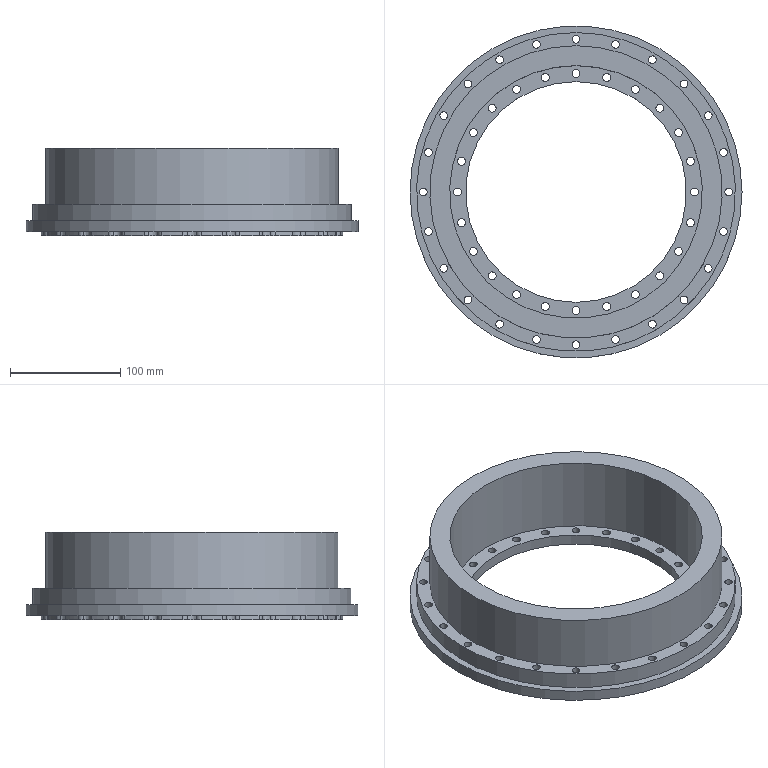Part | STEP file | Inner sleeve | 1 solid | 157 faces | box 301 x 301 x 79.5 mm | volume 1463662 mm3 | cylinder 150 | plane 7 | commonest cylinder face diameters 10 x48 7 x24 7.1 x24 11 x24 274 x24 289 x2